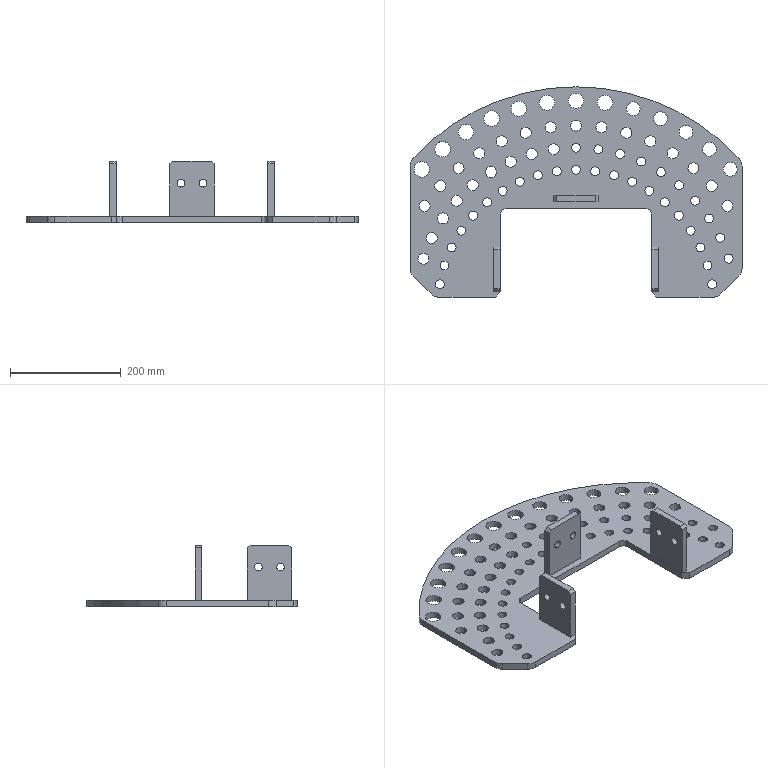Part | SolidWorks | features ICE 7, Chamfer 4, Fillet 2, Extrusion 1 | 4 solids | 194 faces | box 600 x 380 x 112 mm | volume 1912190 mm3 | cylinder 157 | plane 37 | commonest cylinder face diameters 16 x62 20 x50 28 x16 14 x12 25 x10 40 x6